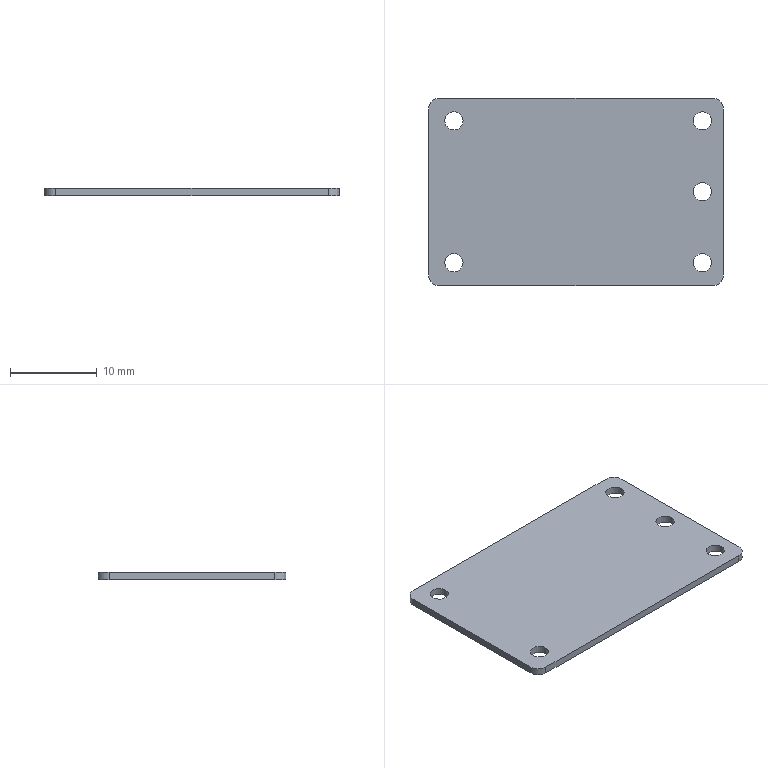Part | STEP file | Driver amplifier PA2PCB | 1 solid | 15 faces | box 34 x 21.66 x 0.832 mm | volume 597.158 mm3 | cylinder 9 | plane 6 | commonest cylinder face diameters 2.1 x5 2.54 x4
STEP:
#1=CARTESIAN_POINT('',(0.,0.,0.));
#2=DIRECTION('',(0.,0.,1.));
#3=DIRECTION('',(1.,0.,0.));
#4=AXIS2_PLACEMENT_3D('',#1,#2,#3);
#5=CARTESIAN_POINT('',(942.668,908.628,0.));
#6=VERTEX_POINT('',#5);
#7=CARTESIAN_POINT('',(942.668,889.508,0.));
#8=VERTEX_POINT('',#7);
#9=CARTESIAN_POINT('',(942.668,908.628,0.));
#10=DIRECTION('',(0.,-1.,0.));
#11=VECTOR('',#10,1.);
#12=LINE('',#9,#11);
#13=CARTESIAN_POINT('',(942.668,908.628,-0.832));
#14=DIRECTION('',(-1.,0.,0.));
#15=DIRECTION('',(0.,0.,1.));
#16=AXIS2_PLACEMENT_3D('',#13,#14,#15);
#17=PLANE('',#16);
#18=CARTESIAN_POINT('',(0.832,0.));
#19=DIRECTION('',(0.,-1.));
#20=VECTOR('',#19,1.);
#21=LINE('',#18,#20);
#22=(GEOMETRIC_REPRESENTATION_CONTEXT(2)PARAMETRIC_REPRESENTATION_CONTEXT()REPRESENTATION_CONTEXT('',''));
#23=DEFINITIONAL_REPRESENTATION('',(#21),#22);
#24=PCURVE('',#17,#23);
#25=CARTESIAN_POINT('',(943.938,889.508,0.));
#26=DIRECTION('',(0.,0.,1.));
#27=DIRECTION('',(1.,0.,0.));
#28=AXIS2_PLACEMENT_3D('',#25,#26,#27);
#29=PLANE('',#28);
#30=CARTESIAN_POINT('',(-1.27,19.12));
#31=DIRECTION('',(0.,-1.));
#32=VECTOR('',#31,1.);
#33=LINE('',#30,#32);
#34=(GEOMETRIC_REPRESENTATION_CONTEXT(2)PARAMETRIC_REPRESENTATION_CONTEXT()REPRESENTATION_CONTEXT('',''));
#35=DEFINITIONAL_REPRESENTATION('',(#33),#34);
#36=PCURVE('',#29,#35);
#37=SURFACE_CURVE('',#12,(#24,#36),.PCURVE_S1.);
#38=EDGE_CURVE('',#6,#8,#37,.T.);
#39=ORIENTED_EDGE('',*,*,#38,.F.);
#40=CARTESIAN_POINT('',(942.668,908.628,-0.832));
#41=VERTEX_POINT('',#40);
#42=CARTESIAN_POINT('',(942.668,908.628,-0.832));
#43=DIRECTION('',(0.,0.,1.));
#44=VECTOR('',#43,1.);
#45=LINE('',#42,#44);
#46=CARTESIAN_POINT('',(0.,0.));
#47=DIRECTION('',(1.,0.));
#48=VECTOR('',#47,1.);
#49=LINE('',#46,#48);
#50=(GEOMETRIC_REPRESENTATION_CONTEXT(2)PARAMETRIC_REPRESENTATION_CONTEXT()REPRESENTATION_CONTEXT('',''));
#51=DEFINITIONAL_REPRESENTATION('',(#49),#50);
#52=PCURVE('',#17,#51);
#53=CARTESIAN_POINT('',(943.938,908.628,-0.832));
#54=DIRECTION('',(0.,0.,1.));
#55=DIRECTION('',(1.,0.,0.));
#56=AXIS2_PLACEMENT_3D('',#53,#54,#55);
#57=CYLINDRICAL_SURFACE('',#56,1.27);
#58=CARTESIAN_POINT('',(3.142,0.));
#59=DIRECTION('',(0.,1.));
#60=VECTOR('',#59,1.);
#61=LINE('',#58,#60);
#62=(GEOMETRIC_REPRESENTATION_CONTEXT(2)PARAMETRIC_REPRESENTATION_CONTEXT()REPRESENTATION_CONTEXT('',''));
#63=DEFINITIONAL_REPRESENTATION('',(#61),#62);
#64=PCURVE('',#57,#63);
#65=SURFACE_CURVE('',#45,(#52,#64),.PCURVE_S1.);
#66=EDGE_CURVE('',#41,#6,#65,.T.);
#67=ORIENTED_EDGE('',*,*,#66,.F.);
#68=CARTESIAN_POINT('',(942.668,889.508,-0.832));
#69=VERTEX_POINT('',#68);
#70=CARTESIAN_POINT('',(942.668,908.628,-0.832));
#71=DIRECTION('',(0.,-1.,0.));
#72=VECTOR('',#71,1.);
#73=LINE('',#70,#72);
#74=CARTESIAN_POINT('',(0.,0.));
#75=DIRECTION('',(0.,-1.));
#76=VECTOR('',#75,1.);
#77=LINE('',#74,#76);
#78=(GEOMETRIC_REPRESENTATION_CONTEXT(2)PARAMETRIC_REPRESENTATION_CONTEXT()REPRESENTATION_CONTEXT('',''));
#79=DEFINITIONAL_REPRESENTATION('',(#77),#78);
#80=PCURVE('',#17,#79);
#81=CARTESIAN_POINT('',(943.938,889.508,-0.832));
#82=DIRECTION('',(0.,0.,1.));
#83=DIRECTION('',(1.,0.,0.));
#84=AXIS2_PLACEMENT_3D('',#81,#82,#83);
#85=PLANE('',#84);
#86=CARTESIAN_POINT('',(-1.27,19.12));
#87=DIRECTION('',(0.,-1.));
#88=VECTOR('',#87,1.);
#89=LINE('',#86,#88);
#90=(GEOMETRIC_REPRESENTATION_CONTEXT(2)PARAMETRIC_REPRESENTATION_CONTEXT()REPRESENTATION_CONTEXT('',''));
#91=DEFINITIONAL_REPRESENTATION('',(#89),#90);
#92=PCURVE('',#85,#91);
#93=SURFACE_CURVE('',#73,(#80,#92),.PCURVE_S1.);
#94=EDGE_CURVE('',#41,#69,#93,.T.);
#95=ORIENTED_EDGE('',*,*,#94,.T.);
#96=CARTESIAN_POINT('',(942.668,889.508,-0.832));
#97=DIRECTION('',(0.,0.,1.));
#98=VECTOR('',#97,1.);
#99=LINE('',#96,#98);
#100=CARTESIAN_POINT('',(0.,-19.12));
#101=DIRECTION('',(1.,0.));
#102=VECTOR('',#101,1.);
#103=LINE('',#100,#102);
#104=(GEOMETRIC_REPRESENTATION_CONTEXT(2)PARAMETRIC_REPRESENTATION_CONTEXT()REPRESENTATION_CONTEXT('',''));
#105=DEFINITIONAL_REPRESENTATION('',(#103),#104);
#106=PCURVE('',#17,#105);
#107=CARTESIAN_POINT('',(943.938,889.508,-0.832));
#108=DIRECTION('',(0.,0.,1.));
#109=DIRECTION('',(1.,0.,0.));
#110=AXIS2_PLACEMENT_3D('',#107,#108,#109);
#111=CYLINDRICAL_SURFACE('',#110,1.27);
#112=CARTESIAN_POINT('',(3.142,0.));
#113=DIRECTION('',(0.,1.));
#114=VECTOR('',#113,1.);
#115=LINE('',#112,#114);
#116=(GEOMETRIC_REPRESENTATION_CONTEXT(2)PARAMETRIC_REPRESENTATION_CONTEXT()REPRESENTATION_CONTEXT('',''));
#117=DEFINITIONAL_REPRESENTATION('',(#115),#116);
#118=PCURVE('',#111,#117);
#119=SURFACE_CURVE('',#99,(#106,#118),.PCURVE_S1.);
#120=EDGE_CURVE('',#69,#8,#119,.T.);
#121=ORIENTED_EDGE('',*,*,#120,.T.);
#122=EDGE_LOOP('',(#39,#67,#95,#121));
#123=FACE_BOUND('',#122,.T.);
#124=ADVANCED_FACE('',(#123),#17,.T.);
#125=CARTESIAN_POINT('',(943.938,888.238,0.));
#126=VERTEX_POINT('',#125);
#127=CARTESIAN_POINT('',(943.938,889.508,0.));
#128=DIRECTION('',(0.,0.,1.));
#129=DIRECTION('',(1.,0.,0.));
#130=AXIS2_PLACEMENT_3D('',#127,#128,#129);
#131=CIRCLE('',#130,1.27);
#132=CARTESIAN_POINT('',(0.,0.832));
#133=DIRECTION('',(1.,0.));
#134=VECTOR('',#133,1.);
#135=LINE('',#132,#134);
#136=(GEOMETRIC_REPRESENTATION_CONTEXT(2)PARAMETRIC_REPRESENTATION_CONTEXT()REPRESENTATION_CONTEXT('',''));
#137=DEFINITIONAL_REPRESENTATION('',(#135),#136);
#138=PCURVE('',#111,#137);
#139=CARTESIAN_POINT('',(0.,0.));
#140=DIRECTION('',(1.,0.));
#141=AXIS2_PLACEMENT_2D('',#139,#140);
#142=CIRCLE('',#141,1.27);
#143=(GEOMETRIC_REPRESENTATION_CONTEXT(2)PARAMETRIC_REPRESENTATION_CONTEXT()REPRESENTATION_CONTEXT('',''));
#144=DEFINITIONAL_REPRESENTATION('',(#142),#143);
#145=PCURVE('',#29,#144);
#146=SURFACE_CURVE('',#131,(#138,#145),.PCURVE_S1.);
#147=EDGE_CURVE('',#8,#126,#146,.T.);
#148=ORIENTED_EDGE('',*,*,#147,.F.);
#149=ORIENTED_EDGE('',*,*,#120,.F.);
#150=CARTESIAN_POINT('',(943.938,888.238,-0.832));
#151=VERTEX_POINT('',#150);
#152=CARTESIAN_POINT('',(943.938,889.508,-0.832));
#153=DIRECTION('',(0.,0.,1.));
#154=DIRECTION('',(1.,0.,0.));
#155=AXIS2_PLACEMENT_3D('',#152,#153,#154);
#156=CIRCLE('',#155,1.27);
#157=CARTESIAN_POINT('',(0.,0.));
#158=DIRECTION('',(1.,0.));
#159=VECTOR('',#158,1.);
#160=LINE('',#157,#159);
#161=(GEOMETRIC_REPRESENTATION_CONTEXT(2)PARAMETRIC_REPRESENTATION_CONTEXT()REPRESENTATION_CONTEXT('',''));
#162=DEFINITIONAL_REPRESENTATION('',(#160),#161);
#163=PCURVE('',#111,#162);
#164=CARTESIAN_POINT('',(0.,0.));
#165=DIRECTION('',(1.,0.));
#166=AXIS2_PLACEMENT_2D('',#164,#165);
#167=CIRCLE('',#166,1.27);
#168=(GEOMETRIC_REPRESENTATION_CONTEXT(2)PARAMETRIC_REPRESENTATION_CONTEXT()REPRESENTATION_CONTEXT('',''));
#169=DEFINITIONAL_REPRESENTATION('',(#167),#168);
#170=PCURVE('',#85,#169);
#171=SURFACE_CURVE('',#156,(#163,#170),.PCURVE_S1.);
#172=EDGE_CURVE('',#69,#151,#171,.T.);
#173=ORIENTED_EDGE('',*,*,#172,.T.);
#174=CARTESIAN_POINT('',(943.938,888.238,-0.832));
#175=DIRECTION('',(0.,0.,1.));
#176=VECTOR('',#175,1.);
#177=LINE('',#174,#176);
#178=CARTESIAN_POINT('',(4.712,0.));
#179=DIRECTION('',(0.,1.));
#180=VECTOR('',#179,1.);
#181=LINE('',#178,#180);
#182=(GEOMETRIC_REPRESENTATION_CONTEXT(2)PARAMETRIC_REPRESENTATION_CONTEXT()REPRESENTATION_CONTEXT('',''));
#183=DEFINITIONAL_REPRESENTATION('',(#181),#182);
#184=PCURVE('',#111,#183);
#185=CARTESIAN_POINT('',(943.938,888.238,-0.832));
#186=DIRECTION('',(0.000000081,-1.,0.));
#187=DIRECTION('',(1.,0.000000081,0.));
#188=AXIS2_PLACEMENT_3D('',#185,#186,#187);
#189=PLANE('',#188);
#190=CARTESIAN_POINT('',(0.,0.));
#191=DIRECTION('',(0.,1.));
#192=VECTOR('',#191,1.);
#193=LINE('',#190,#192);
#194=(GEOMETRIC_REPRESENTATION_CONTEXT(2)PARAMETRIC_REPRESENTATION_CONTEXT()REPRESENTATION_CONTEXT('',''));
#195=DEFINITIONAL_REPRESENTATION('',(#193),#194);
#196=PCURVE('',#189,#195);
#197=SURFACE_CURVE('',#177,(#184,#196),.PCURVE_S1.);
#198=EDGE_CURVE('',#151,#126,#197,.T.);
#199=ORIENTED_EDGE('',*,*,#198,.T.);
#200=EDGE_LOOP('',(#148,#149,#173,#199));
#201=FACE_BOUND('',#200,.T.);
#202=ADVANCED_FACE('',(#201),#111,.T.);
#203=CARTESIAN_POINT('',(975.398,888.238,0.));
#204=VERTEX_POINT('',#203);
#205=CARTESIAN_POINT('',(943.938,888.238,0.));
#206=DIRECTION('',(1.,0.000000081,0.));
#207=VECTOR('',#206,1.);
#208=LINE('',#205,#207);
#209=CARTESIAN_POINT('',(0.,0.832));
#210=DIRECTION('',(1.,0.));
#211=VECTOR('',#210,1.);
#212=LINE('',#209,#211);
#213=(GEOMETRIC_REPRESENTATION_CONTEXT(2)PARAMETRIC_REPRESENTATION_CONTEXT()REPRESENTATION_CONTEXT('',''));
#214=DEFINITIONAL_REPRESENTATION('',(#212),#213);
#215=PCURVE('',#189,#214);
#216=CARTESIAN_POINT('',(0.,-1.27));
#217=DIRECTION('',(1.,0.000000081));
#218=VECTOR('',#217,1.);
#219=LINE('',#216,#218);
#220=(GEOMETRIC_REPRESENTATION_CONTEXT(2)PARAMETRIC_REPRESENTATION_CONTEXT()REPRESENTATION_CONTEXT('',''));
#221=DEFINITIONAL_REPRESENTATION('',(#219),#220);
#222=PCURVE('',#29,#221);
#223=SURFACE_CURVE('',#208,(#215,#222),.PCURVE_S1.);
#224=EDGE_CURVE('',#126,#204,#223,.T.);
#225=ORIENTED_EDGE('',*,*,#224,.F.);
#226=ORIENTED_EDGE('',*,*,#198,.F.);
#227=CARTESIAN_POINT('',(975.398,888.238,-0.832));
#228=VERTEX_POINT('',#227);
#229=CARTESIAN_POINT('',(943.938,888.238,-0.832));
#230=DIRECTION('',(1.,0.000000081,0.));
#231=VECTOR('',#230,1.);
#232=LINE('',#229,#231);
#233=CARTESIAN_POINT('',(0.,0.));
#234=DIRECTION('',(1.,0.));
#235=VECTOR('',#234,1.);
#236=LINE('',#233,#235);
#237=(GEOMETRIC_REPRESENTATION_CONTEXT(2)PARAMETRIC_REPRESENTATION_CONTEXT()REPRESENTATION_CONTEXT('',''));
#238=DEFINITIONAL_REPRESENTATION('',(#236),#237);
#239=PCURVE('',#189,#238);
#240=CARTESIAN_POINT('',(0.,-1.27));
#241=DIRECTION('',(1.,0.000000081));
#242=VECTOR('',#241,1.);
#243=LINE('',#240,#242);
#244=(GEOMETRIC_REPRESENTATION_CONTEXT(2)PARAMETRIC_REPRESENTATION_CONTEXT()REPRESENTATION_CONTEXT('',''));
#245=DEFINITIONAL_REPRESENTATION('',(#243),#244);
#246=PCURVE('',#85,#245);
#247=SURFACE_CURVE('',#232,(#239,#246),.PCURVE_S1.);
#248=EDGE_CURVE('',#151,#228,#247,.T.);
#249=ORIENTED_EDGE('',*,*,#248,.T.);
#250=CARTESIAN_POINT('',(975.398,888.238,-0.832));
#251=DIRECTION('',(0.,0.,1.));
#252=VECTOR('',#251,1.);
#253=LINE('',#250,#252);
#254=CARTESIAN_POINT('',(31.46,0.));
#255=DIRECTION('',(0.,1.));
#256=VECTOR('',#255,1.);
#257=LINE('',#254,#256);
#258=(GEOMETRIC_REPRESENTATION_CONTEXT(2)PARAMETRIC_REPRESENTATION_CONTEXT()REPRESENTATION_CONTEXT('',''));
#259=DEFINITIONAL_REPRESENTATION('',(#257),#258);
#260=PCURVE('',#189,#259);
#261=CARTESIAN_POINT('',(975.398,889.508,-0.832));
#262=DIRECTION('',(0.,0.,1.));
#263=DIRECTION('',(1.,0.,0.));
#264=AXIS2_PLACEMENT_3D('',#261,#262,#263);
#265=CYLINDRICAL_SURFACE('',#264,1.27);
#266=CARTESIAN_POINT('',(4.712,0.));
#267=DIRECTION('',(0.,1.));
#268=VECTOR('',#267,1.);
#269=LINE('',#266,#268);
#270=(GEOMETRIC_REPRESENTATION_CONTEXT(2)PARAMETRIC_REPRESENTATION_CONTEXT()REPRESENTATION_CONTEXT('',''));
#271=DEFINITIONAL_REPRESENTATION('',(#269),#270);
#272=PCURVE('',#265,#271);
#273=SURFACE_CURVE('',#253,(#260,#272),.PCURVE_S1.);
#274=EDGE_CURVE('',#228,#204,#273,.T.);
#275=ORIENTED_EDGE('',*,*,#274,.T.);
#276=EDGE_LOOP('',(#225,#226,#249,#275));
#277=FACE_BOUND('',#276,.T.);
#278=ADVANCED_FACE('',(#277),#189,.T.);
#279=CARTESIAN_POINT('',(976.668,889.508,0.));
#280=VERTEX_POINT('',#279);
#281=CARTESIAN_POINT('',(975.398,889.508,0.));
#282=DIRECTION('',(0.,0.,1.));
#283=DIRECTION('',(1.,0.,0.));
#284=AXIS2_PLACEMENT_3D('',#281,#282,#283);
#285=CIRCLE('',#284,1.27);
#286=CARTESIAN_POINT('',(0.,0.832));
#287=DIRECTION('',(1.,0.));
#288=VECTOR('',#287,1.);
#289=LINE('',#286,#288);
#290=(GEOMETRIC_REPRESENTATION_CONTEXT(2)PARAMETRIC_REPRESENTATION_CONTEXT()REPRESENTATION_CONTEXT('',''));
#291=DEFINITIONAL_REPRESENTATION('',(#289),#290);
#292=PCURVE('',#265,#291);
#293=CARTESIAN_POINT('',(31.46,0.00000254));
#294=DIRECTION('',(1.,0.));
#295=AXIS2_PLACEMENT_2D('',#293,#294);
#296=CIRCLE('',#295,1.27);
#297=(GEOMETRIC_REPRESENTATION_CONTEXT(2)PARAMETRIC_REPRESENTATION_CONTEXT()REPRESENTATION_CONTEXT('',''));
#298=DEFINITIONAL_REPRESENTATION('',(#296),#297);
#299=PCURVE('',#29,#298);
#300=SURFACE_CURVE('',#285,(#292,#299),.PCURVE_S1.);
#301=EDGE_CURVE('',#204,#280,#300,.T.);
#302=ORIENTED_EDGE('',*,*,#301,.F.);
#303=ORIENTED_EDGE('',*,*,#274,.F.);
#304=CARTESIAN_POINT('',(976.668,889.508,-0.832));
#305=VERTEX_POINT('',#304);
#306=CARTESIAN_POINT('',(975.398,889.508,-0.832));
#307=DIRECTION('',(0.,0.,1.));
#308=DIRECTION('',(1.,0.,0.));
#309=AXIS2_PLACEMENT_3D('',#306,#307,#308);
#310=CIRCLE('',#309,1.27);
#311=CARTESIAN_POINT('',(0.,0.));
#312=DIRECTION('',(1.,0.));
#313=VECTOR('',#312,1.);
#314=LINE('',#311,#313);
#315=(GEOMETRIC_REPRESENTATION_CONTEXT(2)PARAMETRIC_REPRESENTATION_CONTEXT()REPRESENTATION_CONTEXT('',''));
#316=DEFINITIONAL_REPRESENTATION('',(#314),#315);
#317=PCURVE('',#265,#316);
#318=CARTESIAN_POINT('',(31.46,0.00000254));
#319=DIRECTION('',(1.,0.));
#320=AXIS2_PLACEMENT_2D('',#318,#319);
#321=CIRCLE('',#320,1.27);
#322=(GEOMETRIC_REPRESENTATION_CONTEXT(2)PARAMETRIC_REPRESENTATION_CONTEXT()REPRESENTATION_CONTEXT('',''));
#323=DEFINITIONAL_REPRESENTATION('',(#321),#322);
#324=PCURVE('',#85,#323);
#325=SURFACE_CURVE('',#310,(#317,#324),.PCURVE_S1.);
#326=EDGE_CURVE('',#228,#305,#325,.T.);
#327=ORIENTED_EDGE('',*,*,#326,.T.);
#328=CARTESIAN_POINT('',(976.668,889.508,-0.832));
#329=DIRECTION('',(0.,0.,1.));
#330=VECTOR('',#329,1.);
#331=LINE('',#328,#330);
#332=CARTESIAN_POINT('',(6.283,0.));
#333=DIRECTION('',(0.,1.));
#334=VECTOR('',#333,1.);
#335=LINE('',#332,#334);
#336=(GEOMETRIC_REPRESENTATION_CONTEXT(2)PARAMETRIC_REPRESENTATION_CONTEXT()REPRESENTATION_CONTEXT('',''));
#337=DEFINITIONAL_REPRESENTATION('',(#335),#336);
#338=PCURVE('',#265,#337);
#339=CARTESIAN_POINT('',(976.668,889.508,-0.832));
#340=DIRECTION('',(1.,0.,0.));
#341=DIRECTION('',(0.,0.,-1.));
#342=AXIS2_PLACEMENT_3D('',#339,#340,#341);
#343=PLANE('',#342);
#344=CARTESIAN_POINT('',(0.,0.));
#345=DIRECTION('',(-1.,0.));
#346=VECTOR('',#345,1.);
#347=LINE('',#344,#346);
#348=(GEOMETRIC_REPRESENTATION_CONTEXT(2)PARAMETRIC_REPRESENTATION_CONTEXT()REPRESENTATION_CONTEXT('',''));
#349=DEFINITIONAL_REPRESENTATION('',(#347),#348);
#350=PCURVE('',#343,#349);
#351=SURFACE_CURVE('',#331,(#338,#350),.PCURVE_S1.);
#352=EDGE_CURVE('',#305,#280,#351,.T.);
#353=ORIENTED_EDGE('',*,*,#352,.T.);
#354=EDGE_LOOP('',(#302,#303,#327,#353));
#355=FACE_BOUND('',#354,.T.);
#356=ADVANCED_FACE('',(#355),#265,.T.);
#357=CARTESIAN_POINT('',(976.668,908.628,0.));
#358=VERTEX_POINT('',#357);
#359=CARTESIAN_POINT('',(976.668,889.508,0.));
#360=DIRECTION('',(0.,1.,0.));
#361=VECTOR('',#360,1.);
#362=LINE('',#359,#361);
#363=CARTESIAN_POINT('',(-0.832,0.));
#364=DIRECTION('',(0.,1.));
#365=VECTOR('',#364,1.);
#366=LINE('',#363,#365);
#367=(GEOMETRIC_REPRESENTATION_CONTEXT(2)PARAMETRIC_REPRESENTATION_CONTEXT()REPRESENTATION_CONTEXT('',''));
#368=DEFINITIONAL_REPRESENTATION('',(#366),#367);
#369=PCURVE('',#343,#368);
#370=CARTESIAN_POINT('',(32.73,0.00000254));
#371=DIRECTION('',(0.,1.));
#372=VECTOR('',#371,1.);
#373=LINE('',#370,#372);
#374=(GEOMETRIC_REPRESENTATION_CONTEXT(2)PARAMETRIC_REPRESENTATION_CONTEXT()REPRESENTATION_CONTEXT('',''));
#375=DEFINITIONAL_REPRESENTATION('',(#373),#374);
#376=PCURVE('',#29,#375);
#377=SURFACE_CURVE('',#362,(#369,#376),.PCURVE_S1.);
#378=EDGE_CURVE('',#280,#358,#377,.T.);
#379=ORIENTED_EDGE('',*,*,#378,.F.);
#380=ORIENTED_EDGE('',*,*,#352,.F.);
#381=CARTESIAN_POINT('',(976.668,908.628,-0.832));
#382=VERTEX_POINT('',#381);
#383=CARTESIAN_POINT('',(976.668,889.508,-0.832));
#384=DIRECTION('',(0.,1.,0.));
#385=VECTOR('',#384,1.);
#386=LINE('',#383,#385);
#387=CARTESIAN_POINT('',(0.,0.));
#388=DIRECTION('',(0.,1.));
#389=VECTOR('',#388,1.);
#390=LINE('',#387,#389);
#391=(GEOMETRIC_REPRESENTATION_CONTEXT(2)PARAMETRIC_REPRESENTATION_CONTEXT()REPRESENTATION_CONTEXT('',''));
#392=DEFINITIONAL_REPRESENTATION('',(#390),#391);
#393=PCURVE('',#343,#392);
#394=CARTESIAN_POINT('',(32.73,0.00000254));
#395=DIRECTION('',(0.,1.));
#396=VECTOR('',#395,1.);
#397=LINE('',#394,#396);
#398=(GEOMETRIC_REPRESENTATION_CONTEXT(2)PARAMETRIC_REPRESENTATION_CONTEXT()REPRESENTATION_CONTEXT('',''));
#399=DEFINITIONAL_REPRESENTATION('',(#397),#398);
#400=PCURVE('',#85,#399);
#401=SURFACE_CURVE('',#386,(#393,#400),.PCURVE_S1.);
#402=EDGE_CURVE('',#305,#382,#401,.T.);
#403=ORIENTED_EDGE('',*,*,#402,.T.);
#404=CARTESIAN_POINT('',(976.668,908.628,-0.832));
#405=DIRECTION('',(0.,0.,1.));
#406=VECTOR('',#405,1.);
#407=LINE('',#404,#406);
#408=CARTESIAN_POINT('',(0.,19.12));
#409=DIRECTION('',(-1.,0.));
#410=VECTOR('',#409,1.);
#411=LINE('',#408,#410);
#412=(GEOMETRIC_REPRESENTATION_CONTEXT(2)PARAMETRIC_REPRESENTATION_CONTEXT()REPRESENTATION_CONTEXT('',''));
#413=DEFINITIONAL_REPRESENTATION('',(#411),#412);
#414=PCURVE('',#343,#413);
#415=CARTESIAN_POINT('',(975.398,908.628,-0.832));
#416=DIRECTION('',(0.,0.,1.));
#417=DIRECTION('',(1.,0.,0.));
#418=AXIS2_PLACEMENT_3D('',#415,#416,#417);
#419=CYLINDRICAL_SURFACE('',#418,1.27);
#420=CARTESIAN_POINT('',(0.,0.));
#421=DIRECTION('',(0.,1.));
#422=VECTOR('',#421,1.);
#423=LINE('',#420,#422);
#424=(GEOMETRIC_REPRESENTATION_CONTEXT(2)PARAMETRIC_REPRESENTATION_CONTEXT()REPRESENTATION_CONTEXT('',''));
#425=DEFINITIONAL_REPRESENTATION('',(#423),#424);
#426=PCURVE('',#419,#425);
#427=SURFACE_CURVE('',#407,(#414,#426),.PCURVE_S1.);
#428=EDGE_CURVE('',#382,#358,#427,.T.);
#429=ORIENTED_EDGE('',*,*,#428,.T.);
#430=EDGE_LOOP('',(#379,#380,#403,#429));
#431=FACE_BOUND('',#430,.T.);
#432=ADVANCED_FACE('',(#431),#343,.T.);
#433=CARTESIAN_POINT('',(975.398,909.898,0.));
#434=VERTEX_POINT('',#433);
#435=CARTESIAN_POINT('',(975.398,908.628,0.));
#436=DIRECTION('',(0.,0.,1.));
#437=DIRECTION('',(1.,0.,0.));
#438=AXIS2_PLACEMENT_3D('',#435,#436,#437);
#439=CIRCLE('',#438,1.27);
#440=CARTESIAN_POINT('',(0.,0.832));
#441=DIRECTION('',(1.,0.));
#442=VECTOR('',#441,1.);
#443=LINE('',#440,#442);
#444=(GEOMETRIC_REPRESENTATION_CONTEXT(2)PARAMETRIC_REPRESENTATION_CONTEXT()REPRESENTATION_CONTEXT('',''));
#445=DEFINITIONAL_REPRESENTATION('',(#443),#444);
#446=PCURVE('',#419,#445);
#447=CARTESIAN_POINT('',(31.46,19.12));
#448=DIRECTION('',(1.,0.));
#449=AXIS2_PLACEMENT_2D('',#447,#448);
#450=CIRCLE('',#449,1.27);
#451=(GEOMETRIC_REPRESENTATION_CONTEXT(2)PARAMETRIC_REPRESENTATION_CONTEXT()REPRESENTATION_CONTEXT('',''));
#452=DEFINITIONAL_REPRESENTATION('',(#450),#451);
#453=PCURVE('',#29,#452);
#454=SURFACE_CURVE('',#439,(#446,#453),.PCURVE_S1.);
#455=EDGE_CURVE('',#358,#434,#454,.T.);
#456=ORIENTED_EDGE('',*,*,#455,.F.);
#457=ORIENTED_EDGE('',*,*,#428,.F.);
#458=CARTESIAN_POINT('',(975.398,909.898,-0.832));
#459=VERTEX_POINT('',#458);
#460=CARTESIAN_POINT('',(975.398,908.628,-0.832));
#461=DIRECTION('',(0.,0.,1.));
#462=DIRECTION('',(1.,0.,0.));
#463=AXIS2_PLACEMENT_3D('',#460,#461,#462);
#464=CIRCLE('',#463,1.27);
#465=CARTESIAN_POINT('',(0.,0.));
#466=DIRECTION('',(1.,0.));
#467=VECTOR('',#466,1.);
#468=LINE('',#465,#467);
#469=(GEOMETRIC_REPRESENTATION_CONTEXT(2)PARAMETRIC_REPRESENTATION_CONTEXT()REPRESENTATION_CONTEXT('',''));
#470=DEFINITIONAL_REPRESENTATION('',(#468),#469);
#471=PCURVE('',#419,#470);
#472=CARTESIAN_POINT('',(31.46,19.12));
#473=DIRECTION('',(1.,0.));
#474=AXIS2_PLACEMENT_2D('',#472,#473);
#475=CIRCLE('',#474,1.27);
#476=(GEOMETRIC_REPRESENTATION_CONTEXT(2)PARAMETRIC_REPRESENTATION_CONTEXT()REPRESENTATION_CONTEXT('',''));
#477=DEFINITIONAL_REPRESENTATION('',(#475),#476);
#478=PCURVE('',#85,#477);
#479=SURFACE_CURVE('',#464,(#471,#478),.PCURVE_S1.);
#480=EDGE_CURVE('',#382,#459,#479,.T.);
#481=ORIENTED_EDGE('',*,*,#480,.T.);
#482=CARTESIAN_POINT('',(975.398,909.898,-0.832));
#483=DIRECTION('',(0.,0.,1.));
#484=VECTOR('',#483,1.);
#485=LINE('',#482,#484);
#486=CARTESIAN_POINT('',(1.571,0.));
#487=DIRECTION('',(0.,1.));
#488=VECTOR('',#487,1.);
#489=LINE('',#486,#488);
#490=(GEOMETRIC_REPRESENTATION_CONTEXT(2)PARAMETRIC_REPRESENTATION_CONTEXT()REPRESENTATION_CONTEXT('',''));
#491=DEFINITIONAL_REPRESENTATION('',(#489),#490);
#492=PCURVE('',#419,#491);
#493=CARTESIAN_POINT('',(975.398,909.898,-0.832));
#494=DIRECTION('',(-0.000000081,1.,0.));
#495=DIRECTION('',(-1.,-0.000000081,0.));
#496=AXIS2_PLACEMENT_3D('',#493,#494,#495);
#497=PLANE('',#496);
#498=CARTESIAN_POINT('',(0.,0.));
#499=DIRECTION('',(0.,1.));
#500=VECTOR('',#499,1.);
#501=LINE('',#498,#500);
#502=(GEOMETRIC_REPRESENTATION_CONTEXT(2)PARAMETRIC_REPRESENTATION_CONTEXT()REPRESENTATION_CONTEXT('',''));
#503=DEFINITIONAL_REPRESENTATION('',(#501),#502);
#504=PCURVE('',#497,#503);
#505=SURFACE_CURVE('',#485,(#492,#504),.PCURVE_S1.);
#506=EDGE_CURVE('',#459,#434,#505,.T.);
#507=ORIENTED_EDGE('',*,*,#506,.T.);
#508=EDGE_LOOP('',(#456,#457,#481,#507));
#509=FACE_BOUND('',#508,.T.);
#510=ADVANCED_FACE('',(#509),#419,.T.);
#511=CARTESIAN_POINT('',(943.938,909.898,0.));
#512=VERTEX_POINT('',#511);
#513=CARTESIAN_POINT('',(975.398,909.898,0.));
#514=DIRECTION('',(-1.,-0.000000081,0.));
#515=VECTOR('',#514,1.);
#516=LINE('',#513,#515);
#517=CARTESIAN_POINT('',(0.,0.832));
#518=DIRECTION('',(1.,0.));
#519=VECTOR('',#518,1.);
#520=LINE('',#517,#519);
#521=(GEOMETRIC_REPRESENTATION_CONTEXT(2)PARAMETRIC_REPRESENTATION_CONTEXT()REPRESENTATION_CONTEXT('',''));
#522=DEFINITIONAL_REPRESENTATION('',(#520),#521);
#523=PCURVE('',#497,#522);
#524=CARTESIAN_POINT('',(31.46,20.39));
#525=DIRECTION('',(-1.,-0.000000081));
#526=VECTOR('',#525,1.);
#527=LINE('',#524,#526);
#528=(GEOMETRIC_REPRESENTATION_CONTEXT(2)PARAMETRIC_REPRESENTATION_CONTEXT()REPRESENTATION_CONTEXT('',''));
#529=DEFINITIONAL_REPRESENTATION('',(#527),#528);
#530=PCURVE('',#29,#529);
#531=SURFACE_CURVE('',#516,(#523,#530),.PCURVE_S1.);
#532=EDGE_CURVE('',#434,#512,#531,.T.);
#533=ORIENTED_EDGE('',*,*,#532,.F.);
#534=ORIENTED_EDGE('',*,*,#506,.F.);
#535=CARTESIAN_POINT('',(943.938,909.898,-0.832));
#536=VERTEX_POINT('',#535);
#537=CARTESIAN_POINT('',(975.398,909.898,-0.832));
#538=DIRECTION('',(-1.,-0.000000081,0.));
#539=VECTOR('',#538,1.);
#540=LINE('',#537,#539);
#541=CARTESIAN_POINT('',(0.,0.));
#542=DIRECTION('',(1.,0.));
#543=VECTOR('',#542,1.);
#544=LINE('',#541,#543);
#545=(GEOMETRIC_REPRESENTATION_CONTEXT(2)PARAMETRIC_REPRESENTATION_CONTEXT()REPRESENTATION_CONTEXT('',''));
#546=DEFINITIONAL_REPRESENTATION('',(#544),#545);
#547=PCURVE('',#497,#546);
#548=CARTESIAN_POINT('',(31.46,20.39));
#549=DIRECTION('',(-1.,-0.000000081));
#550=VECTOR('',#549,1.);
#551=LINE('',#548,#550);
#552=(GEOMETRIC_REPRESENTATION_CONTEXT(2)PARAMETRIC_REPRESENTATION_CONTEXT()REPRESENTATION_CONTEXT('',''));
#553=DEFINITIONAL_REPRESENTATION('',(#551),#552);
#554=PCURVE('',#85,#553);
#555=SURFACE_CURVE('',#540,(#547,#554),.PCURVE_S1.);
#556=EDGE_CURVE('',#459,#536,#555,.T.);
#557=ORIENTED_EDGE('',*,*,#556,.T.);
#558=CARTESIAN_POINT('',(943.938,909.898,-0.832));
#559=DIRECTION('',(0.,0.,1.));
#560=VECTOR('',#559,1.);
#561=LINE('',#558,#560);
#562=CARTESIAN_POINT('',(31.46,0.));
#563=DIRECTION('',(0.,1.));
#564=VECTOR('',#563,1.);
#565=LINE('',#562,#564);
#566=(GEOMETRIC_REPRESENTATION_CONTEXT(2)PARAMETRIC_REPRESENTATION_CONTEXT()REPRESENTATION_CONTEXT('',''));
#567=DEFINITIONAL_REPRESENTATION('',(#565),#566);
#568=PCURVE('',#497,#567);
#569=CARTESIAN_POINT('',(1.571,0.));
#570=DIRECTION('',(0.,1.));
#571=VECTOR('',#570,1.);
#572=LINE('',#569,#571);
#573=(GEOMETRIC_REPRESENTATION_CONTEXT(2)PARAMETRIC_REPRESENTATION_CONTEXT()REPRESENTATION_CONTEXT('',''));
#574=DEFINITIONAL_REPRESENTATION('',(#572),#573);
#575=PCURVE('',#57,#574);
#576=SURFACE_CURVE('',#561,(#568,#575),.PCURVE_S1.);
#577=EDGE_CURVE('',#536,#512,#576,.T.);
#578=ORIENTED_EDGE('',*,*,#577,.T.);
#579=EDGE_LOOP('',(#533,#534,#557,#578));
#580=FACE_BOUND('',#579,.T.);
#581=ADVANCED_FACE('',(#580),#497,.T.);
#582=CARTESIAN_POINT('',(946.638,907.278,-0.832));
#583=VERTEX_POINT('',#582);
#584=CARTESIAN_POINT('',(945.588,907.278,-0.832));
#585=DIRECTION('',(0.,0.,-1.));
#586=DIRECTION('',(1.,0.,0.));
#587=AXIS2_PLACEMENT_3D('',#584,#585,#586);
#588=CIRCLE('',#587,1.05);
#589=CARTESIAN_POINT('',(945.588,907.278,-0.832));
#590=DIRECTION('',(0.,0.,1.));
#591=DIRECTION('',(1.,0.,0.));
#592=AXIS2_PLACEMENT_3D('',#589,#590,#591);
#593=CYLINDRICAL_SURFACE('',#592,1.05);
#594=CARTESIAN_POINT('',(6.283,0.));
#595=DIRECTION('',(-1.,0.));
#596=VECTOR('',#595,1.);
#597=LINE('',#594,#596);
#598=(GEOMETRIC_REPRESENTATION_CONTEXT(2)PARAMETRIC_REPRESENTATION_CONTEXT()REPRESENTATION_CONTEXT('',''));
#599=DEFINITIONAL_REPRESENTATION('',(#597),#598);
#600=PCURVE('',#593,#599);
#601=CARTESIAN_POINT('',(2.7,17.77));
#602=CARTESIAN_POINT('',(2.7,15.951));
#603=CARTESIAN_POINT('',(1.125,16.861));
#604=CARTESIAN_POINT('',(-0.45,17.77));
#605=CARTESIAN_POINT('',(1.125,18.679));
#606=CARTESIAN_POINT('',(2.7,19.589));
#607=CARTESIAN_POINT('',(2.7,17.77));
#608=(BOUNDED_CURVE()B_SPLINE_CURVE(2,(#601,#602,#603,#604,#605,#606,#607),.UNSPECIFIED.,.T.,.F.)B_SPLINE_CURVE_WITH_KNOTS((1,2,2,2,2,1),(-2.094,0.,2.094,4.189,6.283,8.378),.UNSPECIFIED.)CURVE()GEOMETRIC_REPRESENTATION_ITEM()RATIONAL_B_SPLINE_CURVE((1.,0.5,1.,0.5,1.,0.5,1.))REPRESENTATION_ITEM(''));
#609=(GEOMETRIC_REPRESENTATION_CONTEXT(2)PARAMETRIC_REPRESENTATION_CONTEXT()REPRESENTATION_CONTEXT('',''));
#610=DEFINITIONAL_REPRESENTATION('',(#608),#609);
#611=PCURVE('',#85,#610);
#612=SURFACE_CURVE('',#588,(#600,#611),.PCURVE_S1.);
#613=EDGE_CURVE('',#583,#583,#612,.T.);
#614=ORIENTED_EDGE('',*,*,#613,.F.);
#615=CARTESIAN_POINT('',(946.638,907.278,0.));
#616=VERTEX_POINT('',#615);
#617=CARTESIAN_POINT('',(946.638,907.278,-0.832));
#618=CARTESIAN_POINT('',(946.638,907.278,0.));
#619=B_SPLINE_CURVE_WITH_KNOTS('',1,(#617,#618),.UNSPECIFIED.,.F.,.F.,(2,2),(0.,0.832),.PIECEWISE_BEZIER_KNOTS.);
#620=CARTESIAN_POINT('',(6.283,0.));
#621=DIRECTION('',(0.,1.));
#622=VECTOR('',#621,1.);
#623=LINE('',#620,#622);
#624=(GEOMETRIC_REPRESENTATION_CONTEXT(2)PARAMETRIC_REPRESENTATION_CONTEXT()REPRESENTATION_CONTEXT('',''));
#625=DEFINITIONAL_REPRESENTATION('',(#623),#624);
#626=PCURVE('',#593,#625);
#627=CARTESIAN_POINT('',(0.,0.));
#628=DIRECTION('',(0.,1.));
#629=VECTOR('',#628,1.);
#630=LINE('',#627,#629);
#631=(GEOMETRIC_REPRESENTATION_CONTEXT(2)PARAMETRIC_REPRESENTATION_CONTEXT()REPRESENTATION_CONTEXT('',''));
#632=DEFINITIONAL_REPRESENTATION('',(#630),#631);
#633=PCURVE('',#593,#632);
#634=SEAM_CURVE('',#619,(#626,#633),.PCURVE_S1.);
#635=EDGE_CURVE('',#583,#616,#634,.T.);
#636=ORIENTED_EDGE('',*,*,#635,.T.);
#637=CARTESIAN_POINT('',(945.588,907.278,0.));
#638=DIRECTION('',(0.,0.,-1.));
#639=DIRECTION('',(1.,0.,0.));
#640=AXIS2_PLACEMENT_3D('',#637,#638,#639);
#641=CIRCLE('',#640,1.05);
#642=CARTESIAN_POINT('',(6.283,0.832));
#643=DIRECTION('',(-1.,0.));
#644=VECTOR('',#643,1.);
#645=LINE('',#642,#644);
#646=(GEOMETRIC_REPRESENTATION_CONTEXT(2)PARAMETRIC_REPRESENTATION_CONTEXT()REPRESENTATION_CONTEXT('',''));
#647=DEFINITIONAL_REPRESENTATION('',(#645),#646);
#648=PCURVE('',#593,#647);
#649=CARTESIAN_POINT('',(2.7,17.77));
#650=CARTESIAN_POINT('',(2.7,15.951));
#651=CARTESIAN_POINT('',(1.125,16.861));
#652=CARTESIAN_POINT('',(-0.45,17.77));
#653=CARTESIAN_POINT('',(1.125,18.679));
#654=CARTESIAN_POINT('',(2.7,19.589));
#655=CARTESIAN_POINT('',(2.7,17.77));
#656=(BOUNDED_CURVE()B_SPLINE_CURVE(2,(#649,#650,#651,#652,#653,#654,#655),.UNSPECIFIED.,.T.,.F.)B_SPLINE_CURVE_WITH_KNOTS((1,2,2,2,2,1),(-2.094,0.,2.094,4.189,6.283,8.378),.UNSPECIFIED.)CURVE()GEOMETRIC_REPRESENTATION_ITEM()RATIONAL_B_SPLINE_CURVE((1.,0.5,1.,0.5,1.,0.5,1.))REPRESENTATION_ITEM(''));
#657=(GEOMETRIC_REPRESENTATION_CONTEXT(2)PARAMETRIC_REPRESENTATION_CONTEXT()REPRESENTATION_CONTEXT('',''));
#658=DEFINITIONAL_REPRESENTATION('',(#656),#657);
#659=PCURVE('',#29,#658);
#660=SURFACE_CURVE('',#641,(#648,#659),.PCURVE_S1.);
#661=EDGE_CURVE('',#616,#616,#660,.T.);
#662=ORIENTED_EDGE('',*,*,#661,.T.);
#663=ORIENTED_EDGE('',*,*,#635,.F.);
#664=EDGE_LOOP('',(#614,#636,#662,#663));
#665=FACE_BOUND('',#664,.F.);
#666=ADVANCED_FACE('',(#665),#593,.F.);
#667=CARTESIAN_POINT('',(946.638,890.918,-0.832));
#668=VERTEX_POINT('',#667);
#669=CARTESIAN_POINT('',(945.588,890.918,-0.832));
#670=DIRECTION('',(0.,0.,-1.));
#671=DIRECTION('',(1.,0.,0.));
#672=AXIS2_PLACEMENT_3D('',#669,#670,#671);
#673=CIRCLE('',#672,1.05);
#674=CARTESIAN_POINT('',(945.588,890.918,-0.832));
#675=DIRECTION('',(0.,0.,1.));
#676=DIRECTION('',(1.,0.,0.));
#677=AXIS2_PLACEMENT_3D('',#674,#675,#676);
#678=CYLINDRICAL_SURFACE('',#677,1.05);
#679=CARTESIAN_POINT('',(6.283,0.));
#680=DIRECTION('',(-1.,0.));
#681=VECTOR('',#680,1.);
#682=LINE('',#679,#681);
#683=(GEOMETRIC_REPRESENTATION_CONTEXT(2)PARAMETRIC_REPRESENTATION_CONTEXT()REPRESENTATION_CONTEXT('',''));
#684=DEFINITIONAL_REPRESENTATION('',(#682),#683);
#685=PCURVE('',#678,#684);
#686=CARTESIAN_POINT('',(2.7,1.41));
#687=CARTESIAN_POINT('',(2.7,-0.4087));
#688=CARTESIAN_POINT('',(1.125,0.5007));
#689=CARTESIAN_POINT('',(-0.45,1.41));
#690=CARTESIAN_POINT('',(1.125,2.319));
#691=CARTESIAN_POINT('',(2.7,3.229));
#692=CARTESIAN_POINT('',(2.7,1.41));
#693=(BOUNDED_CURVE()B_SPLINE_CURVE(2,(#686,#687,#688,#689,#690,#691,#692),.UNSPECIFIED.,.T.,.F.)B_SPLINE_CURVE_WITH_KNOTS((1,2,2,2,2,1),(-2.094,0.,2.094,4.189,6.283,8.378),.UNSPECIFIED.)CURVE()GEOMETRIC_REPRESENTATION_ITEM()RATIONAL_B_SPLINE_CURVE((1.,0.5,1.,0.5,1.,0.5,1.))REPRESENTATION_ITEM(''));
#694=(GEOMETRIC_REPRESENTATION_CONTEXT(2)PARAMETRIC_REPRESENTATION_CONTEXT()REPRESENTATION_CONTEXT('',''));
#695=DEFINITIONAL_REPRESENTATION('',(#693),#694);
#696=PCURVE('',#85,#695);
#697=SURFACE_CURVE('',#673,(#685,#696),.PCURVE_S1.);
#698=EDGE_CURVE('',#668,#668,#697,.T.);
#699=ORIENTED_EDGE('',*,*,#698,.F.);
#700=CARTESIAN_POINT('',(946.638,890.918,0.));
#701=VERTEX_POINT('',#700);
#702=CARTESIAN_POINT('',(946.638,890.918,-0.832));
#703=CARTESIAN_POINT('',(946.638,890.918,0.));
#704=B_SPLINE_CURVE_WITH_KNOTS('',1,(#702,#703),.UNSPECIFIED.,.F.,.F.,(2,2),(0.,0.832),.PIECEWISE_BEZIER_KNOTS.);
#705=CARTESIAN_POINT('',(6.283,0.));
#706=DIRECTION('',(0.,1.));
#707=VECTOR('',#706,1.);
#708=LINE('',#705,#707);
#709=(GEOMETRIC_REPRESENTATION_CONTEXT(2)PARAMETRIC_REPRESENTATION_CONTEXT()REPRESENTATION_CONTEXT('',''));
#710=DEFINITIONAL_REPRESENTATION('',(#708),#709);
#711=PCURVE('',#678,#710);
#712=CARTESIAN_POINT('',(0.,0.));
#713=DIRECTION('',(0.,1.));
#714=VECTOR('',#713,1.);
#715=LINE('',#712,#714);
#716=(GEOMETRIC_REPRESENTATION_CONTEXT(2)PARAMETRIC_REPRESENTATION_CONTEXT()REPRESENTATION_CONTEXT('',''));
#717=DEFINITIONAL_REPRESENTATION('',(#715),#716);
#718=PCURVE('',#678,#717);
#719=SEAM_CURVE('',#704,(#711,#718),.PCURVE_S1.);
#720=EDGE_CURVE('',#668,#701,#719,.T.);
#721=ORIENTED_EDGE('',*,*,#720,.T.);
#722=CARTESIAN_POINT('',(945.588,890.918,0.));
#723=DIRECTION('',(0.,0.,-1.));
#724=DIRECTION('',(1.,0.,0.));
#725=AXIS2_PLACEMENT_3D('',#722,#723,#724);
#726=CIRCLE('',#725,1.05);
#727=CARTESIAN_POINT('',(6.283,0.832));
#728=DIRECTION('',(-1.,0.));
#729=VECTOR('',#728,1.);
#730=LINE('',#727,#729);
#731=(GEOMETRIC_REPRESENTATION_CONTEXT(2)PARAMETRIC_REPRESENTATION_CONTEXT()REPRESENTATION_CONTEXT('',''));
#732=DEFINITIONAL_REPRESENTATION('',(#730),#731);
#733=PCURVE('',#678,#732);
#734=CARTESIAN_POINT('',(2.7,1.41));
#735=CARTESIAN_POINT('',(2.7,-0.4087));
#736=CARTESIAN_POINT('',(1.125,0.5007));
#737=CARTESIAN_POINT('',(-0.45,1.41));
#738=CARTESIAN_POINT('',(1.125,2.319));
#739=CARTESIAN_POINT('',(2.7,3.229));
#740=CARTESIAN_POINT('',(2.7,1.41));
#741=(BOUNDED_CURVE()B_SPLINE_CURVE(2,(#734,#735,#736,#737,#738,#739,#740),.UNSPECIFIED.,.T.,.F.)B_SPLINE_CURVE_WITH_KNOTS((1,2,2,2,2,1),(-2.094,0.,2.094,4.189,6.283,8.378),.UNSPECIFIED.)CURVE()GEOMETRIC_REPRESENTATION_ITEM()RATIONAL_B_SPLINE_CURVE((1.,0.5,1.,0.5,1.,0.5,1.))REPRESENTATION_ITEM(''));
#742=(GEOMETRIC_REPRESENTATION_CONTEXT(2)PARAMETRIC_REPRESENTATION_CONTEXT()REPRESENTATION_CONTEXT('',''));
#743=DEFINITIONAL_REPRESENTATION('',(#741),#742);
#744=PCURVE('',#29,#743);
#745=SURFACE_CURVE('',#726,(#733,#744),.PCURVE_S1.);
#746=EDGE_CURVE('',#701,#701,#745,.T.);
#747=ORIENTED_EDGE('',*,*,#746,.T.);
#748=ORIENTED_EDGE('',*,*,#720,.F.);
#749=EDGE_LOOP('',(#699,#721,#747,#748));
#750=FACE_BOUND('',#749,.F.);
#751=ADVANCED_FACE('',(#750),#678,.F.);
#752=CARTESIAN_POINT('',(975.278,890.918,-0.832));
#753=VERTEX_POINT('',#752);
#754=CARTESIAN_POINT('',(974.228,890.918,-0.832));
#755=DIRECTION('',(0.,0.,-1.));
#756=DIRECTION('',(1.,0.,0.));
#757=AXIS2_PLACEMENT_3D('',#754,#755,#756);
#758=CIRCLE('',#757,1.05);
#759=CARTESIAN_POINT('',(974.228,890.918,-0.832));
#760=DIRECTION('',(0.,0.,1.));
#761=DIRECTION('',(1.,0.,0.));
#762=AXIS2_PLACEMENT_3D('',#759,#760,#761);
#763=CYLINDRICAL_SURFACE('',#762,1.05);
#764=CARTESIAN_POINT('',(6.283,0.));
#765=DIRECTION('',(-1.,0.));
#766=VECTOR('',#765,1.);
#767=LINE('',#764,#766);
#768=(GEOMETRIC_REPRESENTATION_CONTEXT(2)PARAMETRIC_REPRESENTATION_CONTEXT()REPRESENTATION_CONTEXT('',''));
#769=DEFINITIONAL_REPRESENTATION('',(#767),#768);
#770=PCURVE('',#763,#769);
#771=CARTESIAN_POINT('',(31.34,1.41));
#772=CARTESIAN_POINT('',(31.34,-0.4087));
#773=CARTESIAN_POINT('',(29.765,0.5007));
#774=CARTESIAN_POINT('',(28.19,1.41));
#775=CARTESIAN_POINT('',(29.765,2.319));
#776=CARTESIAN_POINT('',(31.34,3.229));
#777=CARTESIAN_POINT('',(31.34,1.41));
#778=(BOUNDED_CURVE()B_SPLINE_CURVE(2,(#771,#772,#773,#774,#775,#776,#777),.UNSPECIFIED.,.T.,.F.)B_SPLINE_CURVE_WITH_KNOTS((1,2,2,2,2,1),(-2.094,0.,2.094,4.189,6.283,8.378),.UNSPECIFIED.)CURVE()GEOMETRIC_REPRESENTATION_ITEM()RATIONAL_B_SPLINE_CURVE((1.,0.5,1.,0.5,1.,0.5,1.))REPRESENTATION_ITEM(''));
#779=(GEOMETRIC_REPRESENTATION_CONTEXT(2)PARAMETRIC_REPRESENTATION_CONTEXT()REPRESENTATION_CONTEXT('',''));
#780=DEFINITIONAL_REPRESENTATION('',(#778),#779);
#781=PCURVE('',#85,#780);
#782=SURFACE_CURVE('',#758,(#770,#781),.PCURVE_S1.);
#783=EDGE_CURVE('',#753,#753,#782,.T.);
#784=ORIENTED_EDGE('',*,*,#783,.F.);
#785=CARTESIAN_POINT('',(975.278,890.918,0.));
#786=VERTEX_POINT('',#785);
#787=CARTESIAN_POINT('',(975.278,890.918,-0.832));
#788=CARTESIAN_POINT('',(975.278,890.918,0.));
#789=B_SPLINE_CURVE_WITH_KNOTS('',1,(#787,#788),.UNSPECIFIED.,.F.,.F.,(2,2),(0.,0.832),.PIECEWISE_BEZIER_KNOTS.);
#790=CARTESIAN_POINT('',(6.283,0.));
#791=DIRECTION('',(0.,1.));
#792=VECTOR('',#791,1.);
#793=LINE('',#790,#792);
#794=(GEOMETRIC_REPRESENTATION_CONTEXT(2)PARAMETRIC_REPRESENTATION_CONTEXT()REPRESENTATION_CONTEXT('',''));
#795=DEFINITIONAL_REPRESENTATION('',(#793),#794);
#796=PCURVE('',#763,#795);
#797=CARTESIAN_POINT('',(0.,0.));
#798=DIRECTION('',(0.,1.));
#799=VECTOR('',#798,1.);
#800=LINE('',#797,#799);
#801=(GEOMETRIC_REPRESENTATION_CONTEXT(2)PARAMETRIC_REPRESENTATION_CONTEXT()REPRESENTATION_CONTEXT('',''));
#802=DEFINITIONAL_REPRESENTATION('',(#800),#801);
#803=PCURVE('',#763,#802);
#804=SEAM_CURVE('',#789,(#796,#803),.PCURVE_S1.);
#805=EDGE_CURVE('',#753,#786,#804,.T.);
#806=ORIENTED_EDGE('',*,*,#805,.T.);
#807=CARTESIAN_POINT('',(974.228,890.918,0.));
#808=DIRECTION('',(0.,0.,-1.));
#809=DIRECTION('',(1.,0.,0.));
#810=AXIS2_PLACEMENT_3D('',#807,#808,#809);
#811=CIRCLE('',#810,1.05);
#812=CARTESIAN_POINT('',(6.283,0.832));
#813=DIRECTION('',(-1.,0.));
#814=VECTOR('',#813,1.);
#815=LINE('',#812,#814);
#816=(GEOMETRIC_REPRESENTATION_CONTEXT(2)PARAMETRIC_REPRESENTATION_CONTEXT()REPRESENTATION_CONTEXT('',''));
#817=DEFINITIONAL_REPRESENTATION('',(#815),#816);
#818=PCURVE('',#763,#817);
#819=CARTESIAN_POINT('',(31.34,1.41));
#820=CARTESIAN_POINT('',(31.34,-0.4087));
#821=CARTESIAN_POINT('',(29.765,0.5007));
#822=CARTESIAN_POINT('',(28.19,1.41));
#823=CARTESIAN_POINT('',(29.765,2.319));
#824=CARTESIAN_POINT('',(31.34,3.229));
#825=CARTESIAN_POINT('',(31.34,1.41));
#826=(BOUNDED_CURVE()B_SPLINE_CURVE(2,(#819,#820,#821,#822,#823,#824,#825),.UNSPECIFIED.,.T.,.F.)B_SPLINE_CURVE_WITH_KNOTS((1,2,2,2,2,1),(-2.094,0.,2.094,4.189,6.283,8.378),.UNSPECIFIED.)CURVE()GEOMETRIC_REPRESENTATION_ITEM()RATIONAL_B_SPLINE_CURVE((1.,0.5,1.,0.5,1.,0.5,1.))REPRESENTATION_ITEM(''));
#827=(GEOMETRIC_REPRESENTATION_CONTEXT(2)PARAMETRIC_REPRESENTATION_CONTEXT()REPRESENTATION_CONTEXT('',''));
#828=DEFINITIONAL_REPRESENTATION('',(#826),#827);
#829=PCURVE('',#29,#828);
#830=SURFACE_CURVE('',#811,(#818,#829),.PCURVE_S1.);
#831=EDGE_CURVE('',#786,#786,#830,.T.);
#832=ORIENTED_EDGE('',*,*,#831,.T.);
#833=ORIENTED_EDGE('',*,*,#805,.F.);
#834=EDGE_LOOP('',(#784,#806,#832,#833));
#835=FACE_BOUND('',#834,.F.);
#836=ADVANCED_FACE('',(#835),#763,.F.);
#837=CARTESIAN_POINT('',(975.278,907.278,-0.832));
#838=VERTEX_POINT('',#837);
#839=CARTESIAN_POINT('',(974.228,907.278,-0.832));
#840=DIRECTION('',(0.,0.,-1.));
#841=DIRECTION('',(1.,0.,0.));
#842=AXIS2_PLACEMENT_3D('',#839,#840,#841);
#843=CIRCLE('',#842,1.05);
#844=CARTESIAN_POINT('',(974.228,907.278,-0.832));
#845=DIRECTION('',(0.,0.,1.));
#846=DIRECTION('',(1.,0.,0.));
#847=AXIS2_PLACEMENT_3D('',#844,#845,#846);
#848=CYLINDRICAL_SURFACE('',#847,1.05);
#849=CARTESIAN_POINT('',(6.283,0.));
#850=DIRECTION('',(-1.,0.));
#851=VECTOR('',#850,1.);
#852=LINE('',#849,#851);
#853=(GEOMETRIC_REPRESENTATION_CONTEXT(2)PARAMETRIC_REPRESENTATION_CONTEXT()REPRESENTATION_CONTEXT('',''));
#854=DEFINITIONAL_REPRESENTATION('',(#852),#853);
#855=PCURVE('',#848,#854);
#856=CARTESIAN_POINT('',(31.34,17.77));
#857=CARTESIAN_POINT('',(31.34,15.951));
#858=CARTESIAN_POINT('',(29.765,16.861));
#859=CARTESIAN_POINT('',(28.19,17.77));
#860=CARTESIAN_POINT('',(29.765,18.679));
#861=CARTESIAN_POINT('',(31.34,19.589));
#862=CARTESIAN_POINT('',(31.34,17.77));
#863=(BOUNDED_CURVE()B_SPLINE_CURVE(2,(#856,#857,#858,#859,#860,#861,#862),.UNSPECIFIED.,.T.,.F.)B_SPLINE_CURVE_WITH_KNOTS((1,2,2,2,2,1),(-2.094,0.,2.094,4.189,6.283,8.378),.UNSPECIFIED.)CURVE()GEOMETRIC_REPRESENTATION_ITEM()RATIONAL_B_SPLINE_CURVE((1.,0.5,1.,0.5,1.,0.5,1.))REPRESENTATION_ITEM(''));
#864=(GEOMETRIC_REPRESENTATION_CONTEXT(2)PARAMETRIC_REPRESENTATION_CONTEXT()REPRESENTATION_CONTEXT('',''));
#865=DEFINITIONAL_REPRESENTATION('',(#863),#864);
#866=PCURVE('',#85,#865);
#867=SURFACE_CURVE('',#843,(#855,#866),.PCURVE_S1.);
#868=EDGE_CURVE('',#838,#838,#867,.T.);
#869=ORIENTED_EDGE('',*,*,#868,.F.);
#870=CARTESIAN_POINT('',(975.278,907.278,0.));
#871=VERTEX_POINT('',#870);
#872=CARTESIAN_POINT('',(975.278,907.278,-0.832));
#873=CARTESIAN_POINT('',(975.278,907.278,0.));
#874=B_SPLINE_CURVE_WITH_KNOTS('',1,(#872,#873),.UNSPECIFIED.,.F.,.F.,(2,2),(0.,0.832),.PIECEWISE_BEZIER_KNOTS.);
#875=CARTESIAN_POINT('',(6.283,0.));
#876=DIRECTION('',(0.,1.));
#877=VECTOR('',#876,1.);
#878=LINE('',#875,#877);
#879=(GEOMETRIC_REPRESENTATION_CONTEXT(2)PARAMETRIC_REPRESENTATION_CONTEXT()REPRESENTATION_CONTEXT('',''));
#880=DEFINITIONAL_REPRESENTATION('',(#878),#879);
#881=PCURVE('',#848,#880);
#882=CARTESIAN_POINT('',(0.,0.));
#883=DIRECTION('',(0.,1.));
#884=VECTOR('',#883,1.);
#885=LINE('',#882,#884);
#886=(GEOMETRIC_REPRESENTATION_CONTEXT(2)PARAMETRIC_REPRESENTATION_CONTEXT()REPRESENTATION_CONTEXT('',''));
#887=DEFINITIONAL_REPRESENTATION('',(#885),#886);
#888=PCURVE('',#848,#887);
#889=SEAM_CURVE('',#874,(#881,#888),.PCURVE_S1.);
#890=EDGE_CURVE('',#838,#871,#889,.T.);
#891=ORIENTED_EDGE('',*,*,#890,.T.);
#892=CARTESIAN_POINT('',(974.228,907.278,0.));
#893=DIRECTION('',(0.,0.,-1.));
#894=DIRECTION('',(1.,0.,0.));
#895=AXIS2_PLACEMENT_3D('',#892,#893,#894);
#896=CIRCLE('',#895,1.05);
#897=CARTESIAN_POINT('',(6.283,0.832));
#898=DIRECTION('',(-1.,0.));
#899=VECTOR('',#898,1.);
#900=LINE('',#897,#899);
#901=(GEOMETRIC_REPRESENTATION_CONTEXT(2)PARAMETRIC_REPRESENTATION_CONTEXT()REPRESENTATION_CONTEXT('',''));
#902=DEFINITIONAL_REPRESENTATION('',(#900),#901);
#903=PCURVE('',#848,#902);
#904=CARTESIAN_POINT('',(31.34,17.77));
#905=CARTESIAN_POINT('',(31.34,15.951));
#906=CARTESIAN_POINT('',(29.765,16.861));
#907=CARTESIAN_POINT('',(28.19,17.77));
#908=CARTESIAN_POINT('',(29.765,18.679));
#909=CARTESIAN_POINT('',(31.34,19.589));
#910=CARTESIAN_POINT('',(31.34,17.77));
#911=(BOUNDED_CURVE()B_SPLINE_CURVE(2,(#904,#905,#906,#907,#908,#909,#910),.UNSPECIFIED.,.T.,.F.)B_SPLINE_CURVE_WITH_KNOTS((1,2,2,2,2,1),(-2.094,0.,2.094,4.189,6.283,8.378),.UNSPECIFIED.)CURVE()GEOMETRIC_REPRESENTATION_ITEM()RATIONAL_B_SPLINE_CURVE((1.,0.5,1.,0.5,1.,0.5,1.))REPRESENTATION_ITEM(''));
#912=(GEOMETRIC_REPRESENTATION_CONTEXT(2)PARAMETRIC_REPRESENTATION_CONTEXT()REPRESENTATION_CONTEXT('',''));
#913=DEFINITIONAL_REPRESENTATION('',(#911),#912);
#914=PCURVE('',#29,#913);
#915=SURFACE_CURVE('',#896,(#903,#914),.PCURVE_S1.);
#916=EDGE_CURVE('',#871,#871,#915,.T.);
#917=ORIENTED_EDGE('',*,*,#916,.T.);
#918=ORIENTED_EDGE('',*,*,#890,.F.);
#919=EDGE_LOOP('',(#869,#891,#917,#918));
#920=FACE_BOUND('',#919,.F.);
#921=ADVANCED_FACE('',(#920),#848,.F.);
#922=CARTESIAN_POINT('',(943.938,908.628,0.));
#923=DIRECTION('',(0.,0.,1.));
#924=DIRECTION('',(1.,0.,0.));
#925=AXIS2_PLACEMENT_3D('',#922,#923,#924);
#926=CIRCLE('',#925,1.27);
#927=CARTESIAN_POINT('',(0.,0.832));
#928=DIRECTION('',(1.,0.));
#929=VECTOR('',#928,1.);
#930=LINE('',#927,#929);
#931=(GEOMETRIC_REPRESENTATION_CONTEXT(2)PARAMETRIC_REPRESENTATION_CONTEXT()REPRESENTATION_CONTEXT('',''));
#932=DEFINITIONAL_REPRESENTATION('',(#930),#931);
#933=PCURVE('',#57,#932);
#934=CARTESIAN_POINT('',(0.,19.12));
#935=DIRECTION('',(1.,0.));
#936=AXIS2_PLACEMENT_2D('',#934,#935);
#937=CIRCLE('',#936,1.27);
#938=(GEOMETRIC_REPRESENTATION_CONTEXT(2)PARAMETRIC_REPRESENTATION_CONTEXT()REPRESENTATION_CONTEXT('',''));
#939=DEFINITIONAL_REPRESENTATION('',(#937),#938);
#940=PCURVE('',#29,#939);
#941=SURFACE_CURVE('',#926,(#933,#940),.PCURVE_S1.);
#942=EDGE_CURVE('',#512,#6,#941,.T.);
#943=ORIENTED_EDGE('',*,*,#942,.F.);
#944=ORIENTED_EDGE('',*,*,#577,.F.);
#945=CARTESIAN_POINT('',(943.938,908.628,-0.832));
#946=DIRECTION('',(0.,0.,1.));
#947=DIRECTION('',(1.,0.,0.));
#948=AXIS2_PLACEMENT_3D('',#945,#946,#947);
#949=CIRCLE('',#948,1.27);
#950=CARTESIAN_POINT('',(0.,0.));
#951=DIRECTION('',(1.,0.));
#952=VECTOR('',#951,1.);
#953=LINE('',#950,#952);
#954=(GEOMETRIC_REPRESENTATION_CONTEXT(2)PARAMETRIC_REPRESENTATION_CONTEXT()REPRESENTATION_CONTEXT('',''));
#955=DEFINITIONAL_REPRESENTATION('',(#953),#954);
#956=PCURVE('',#57,#955);
#957=CARTESIAN_POINT('',(0.,19.12));
#958=DIRECTION('',(1.,0.));
#959=AXIS2_PLACEMENT_2D('',#957,#958);
#960=CIRCLE('',#959,1.27);
#961=(GEOMETRIC_REPRESENTATION_CONTEXT(2)PARAMETRIC_REPRESENTATION_CONTEXT()REPRESENTATION_CONTEXT('',''));
#962=DEFINITIONAL_REPRESENTATION('',(#960),#961);
#963=PCURVE('',#85,#962);
#964=SURFACE_CURVE('',#949,(#956,#963),.PCURVE_S1.);
#965=EDGE_CURVE('',#536,#41,#964,.T.);
#966=ORIENTED_EDGE('',*,*,#965,.T.);
#967=ORIENTED_EDGE('',*,*,#66,.T.);
#968=EDGE_LOOP('',(#943,#944,#966,#967));
#969=FACE_BOUND('',#968,.T.);
#970=ADVANCED_FACE('',(#969),#57,.T.);
#971=CARTESIAN_POINT('',(975.278,899.098,-0.832));
#972=VERTEX_POINT('',#971);
#973=CARTESIAN_POINT('',(974.228,899.098,-0.832));
#974=DIRECTION('',(0.,0.,-1.));
#975=DIRECTION('',(1.,0.,0.));
#976=AXIS2_PLACEMENT_3D('',#973,#974,#975);
#977=CIRCLE('',#976,1.05);
#978=CARTESIAN_POINT('',(974.228,899.098,-0.832));
#979=DIRECTION('',(0.,0.,1.));
#980=DIRECTION('',(1.,0.,0.));
#981=AXIS2_PLACEMENT_3D('',#978,#979,#980);
#982=CYLINDRICAL_SURFACE('',#981,1.05);
#983=CARTESIAN_POINT('',(6.283,0.));
#984=DIRECTION('',(-1.,0.));
#985=VECTOR('',#984,1.);
#986=LINE('',#983,#985);
#987=(GEOMETRIC_REPRESENTATION_CONTEXT(2)PARAMETRIC_REPRESENTATION_CONTEXT()REPRESENTATION_CONTEXT('',''));
#988=DEFINITIONAL_REPRESENTATION('',(#986),#987);
#989=PCURVE('',#982,#988);
#990=CARTESIAN_POINT('',(31.34,9.59));
#991=CARTESIAN_POINT('',(31.34,7.771));
#992=CARTESIAN_POINT('',(29.765,8.681));
#993=CARTESIAN_POINT('',(28.19,9.59));
#994=CARTESIAN_POINT('',(29.765,10.499));
#995=CARTESIAN_POINT('',(31.34,11.409));
#996=CARTESIAN_POINT('',(31.34,9.59));
#997=(BOUNDED_CURVE()B_SPLINE_CURVE(2,(#990,#991,#992,#993,#994,#995,#996),.UNSPECIFIED.,.T.,.F.)B_SPLINE_CURVE_WITH_KNOTS((1,2,2,2,2,1),(-2.094,0.,2.094,4.189,6.283,8.378),.UNSPECIFIED.)CURVE()GEOMETRIC_REPRESENTATION_ITEM()RATIONAL_B_SPLINE_CURVE((1.,0.5,1.,0.5,1.,0.5,1.))REPRESENTATION_ITEM(''));
#998=(GEOMETRIC_REPRESENTATION_CONTEXT(2)PARAMETRIC_REPRESENTATION_CONTEXT()REPRESENTATION_CONTEXT('',''));
#999=DEFINITIONAL_REPRESENTATION('',(#997),#998);
#1000=PCURVE('',#85,#999);
#1001=SURFACE_CURVE('',#977,(#989,#1000),.PCURVE_S1.);
#1002=EDGE_CURVE('',#972,#972,#1001,.T.);
#1003=ORIENTED_EDGE('',*,*,#1002,.F.);
#1004=CARTESIAN_POINT('',(975.278,899.098,0.));
#1005=VERTEX_POINT('',#1004);
#1006=CARTESIAN_POINT('',(975.278,899.098,-0.832));
#1007=CARTESIAN_POINT('',(975.278,899.098,0.));
#1008=B_SPLINE_CURVE_WITH_KNOTS('',1,(#1006,#1007),.UNSPECIFIED.,.F.,.F.,(2,2),(0.,0.832),.PIECEWISE_BEZIER_KNOTS.);
#1009=CARTESIAN_POINT('',(6.283,0.));
#1010=DIRECTION('',(0.,1.));
#1011=VECTOR('',#1010,1.);
#1012=LINE('',#1009,#1011);
#1013=(GEOMETRIC_REPRESENTATION_CONTEXT(2)PARAMETRIC_REPRESENTATION_CONTEXT()REPRESENTATION_CONTEXT('',''));
#1014=DEFINITIONAL_REPRESENTATION('',(#1012),#1013);
#1015=PCURVE('',#982,#1014);
#1016=CARTESIAN_POINT('',(0.,0.));
#1017=DIRECTION('',(0.,1.));
#1018=VECTOR('',#1017,1.);
#1019=LINE('',#1016,#1018);
#1020=(GEOMETRIC_REPRESENTATION_CONTEXT(2)PARAMETRIC_REPRESENTATION_CONTEXT()REPRESENTATION_CONTEXT('',''));
#1021=DEFINITIONAL_REPRESENTATION('',(#1019),#1020);
#1022=PCURVE('',#982,#1021);
#1023=SEAM_CURVE('',#1008,(#1015,#1022),.PCURVE_S1.);
#1024=EDGE_CURVE('',#972,#1005,#1023,.T.);
#1025=ORIENTED_EDGE('',*,*,#1024,.T.);
#1026=CARTESIAN_POINT('',(974.228,899.098,0.));
#1027=DIRECTION('',(0.,0.,-1.));
#1028=DIRECTION('',(1.,0.,0.));
#1029=AXIS2_PLACEMENT_3D('',#1026,#1027,#1028);
#1030=CIRCLE('',#1029,1.05);
#1031=CARTESIAN_POINT('',(6.283,0.832));
#1032=DIRECTION('',(-1.,0.));
#1033=VECTOR('',#1032,1.);
#1034=LINE('',#1031,#1033);
#1035=(GEOMETRIC_REPRESENTATION_CONTEXT(2)PARAMETRIC_REPRESENTATION_CONTEXT()REPRESENTATION_CONTEXT('',''));
#1036=DEFINITIONAL_REPRESENTATION('',(#1034),#1035);
#1037=PCURVE('',#982,#1036);
#1038=CARTESIAN_POINT('',(31.34,9.59));
#1039=CARTESIAN_POINT('',(31.34,7.771));
#1040=CARTESIAN_POINT('',(29.765,8.681));
#1041=CARTESIAN_POINT('',(28.19,9.59));
#1042=CARTESIAN_POINT('',(29.765,10.499));
#1043=CARTESIAN_POINT('',(31.34,11.409));
#1044=CARTESIAN_POINT('',(31.34,9.59));
#1045=(BOUNDED_CURVE()B_SPLINE_CURVE(2,(#1038,#1039,#1040,#1041,#1042,#1043,#1044),.UNSPECIFIED.,.T.,.F.)B_SPLINE_CURVE_WITH_KNOTS((1,2,2,2,2,1),(-2.094,0.,2.094,4.189,6.283,8.378),.UNSPECIFIED.)CURVE()GEOMETRIC_REPRESENTATION_ITEM()RATIONAL_B_SPLINE_CURVE((1.,0.5,1.,0.5,1.,0.5,1.))REPRESENTATION_ITEM(''));
#1046=(GEOMETRIC_REPRESENTATION_CONTEXT(2)PARAMETRIC_REPRESENTATION_CONTEXT()REPRESENTATION_CONTEXT('',''));
#1047=DEFINITIONAL_REPRESENTATION('',(#1045),#1046);
#1048=PCURVE('',#29,#1047);
#1049=SURFACE_CURVE('',#1030,(#1037,#1048),.PCURVE_S1.);
#1050=EDGE_CURVE('',#1005,#1005,#1049,.T.);
#1051=ORIENTED_EDGE('',*,*,#1050,.T.);
#1052=ORIENTED_EDGE('',*,*,#1024,.F.);
#1053=EDGE_LOOP('',(#1003,#1025,#1051,#1052));
#1054=FACE_BOUND('',#1053,.F.);
#1055=ADVANCED_FACE('',(#1054),#982,.F.);
#1056=ORIENTED_EDGE('',*,*,#94,.F.);
#1057=ORIENTED_EDGE('',*,*,#965,.F.);
#1058=ORIENTED_EDGE('',*,*,#556,.F.);
#1059=ORIENTED_EDGE('',*,*,#480,.F.);
#1060=ORIENTED_EDGE('',*,*,#402,.F.);
#1061=ORIENTED_EDGE('',*,*,#326,.F.);
#1062=ORIENTED_EDGE('',*,*,#248,.F.);
#1063=ORIENTED_EDGE('',*,*,#172,.F.);
#1064=EDGE_LOOP('',(#1056,#1057,#1058,#1059,#1060,#1061,#1062,#1063));
#1065=FACE_BOUND('',#1064,.T.);
#1066=ORIENTED_EDGE('',*,*,#868,.F.);
#1067=EDGE_LOOP('',(#1066));
#1068=FACE_BOUND('',#1067,.T.);
#1069=ORIENTED_EDGE('',*,*,#783,.F.);
#1070=EDGE_LOOP('',(#1069));
#1071=FACE_BOUND('',#1070,.T.);
#1072=ORIENTED_EDGE('',*,*,#698,.F.);
#1073=EDGE_LOOP('',(#1072));
#1074=FACE_BOUND('',#1073,.T.);
#1075=ORIENTED_EDGE('',*,*,#613,.F.);
#1076=EDGE_LOOP('',(#1075));
#1077=FACE_BOUND('',#1076,.T.);
#1078=ORIENTED_EDGE('',*,*,#1002,.F.);
#1079=EDGE_LOOP('',(#1078));
#1080=FACE_BOUND('',#1079,.T.);
#1081=ADVANCED_FACE('',(#1065,#1068,#1071,#1074,#1077,#1080),#85,.F.);
#1082=ORIENTED_EDGE('',*,*,#38,.T.);
#1083=ORIENTED_EDGE('',*,*,#147,.T.);
#1084=ORIENTED_EDGE('',*,*,#224,.T.);
#1085=ORIENTED_EDGE('',*,*,#301,.T.);
#1086=ORIENTED_EDGE('',*,*,#378,.T.);
#1087=ORIENTED_EDGE('',*,*,#455,.T.);
#1088=ORIENTED_EDGE('',*,*,#532,.T.);
#1089=ORIENTED_EDGE('',*,*,#942,.T.);
#1090=EDGE_LOOP('',(#1082,#1083,#1084,#1085,#1086,#1087,#1088,#1089));
#1091=FACE_BOUND('',#1090,.T.);
#1092=ORIENTED_EDGE('',*,*,#916,.T.);
#1093=EDGE_LOOP('',(#1092));
#1094=FACE_BOUND('',#1093,.T.);
#1095=ORIENTED_EDGE('',*,*,#831,.T.);
#1096=EDGE_LOOP('',(#1095));
#1097=FACE_BOUND('',#1096,.T.);
#1098=ORIENTED_EDGE('',*,*,#746,.T.);
#1099=EDGE_LOOP('',(#1098));
#1100=FACE_BOUND('',#1099,.T.);
#1101=ORIENTED_EDGE('',*,*,#661,.T.);
#1102=EDGE_LOOP('',(#1101));
#1103=FACE_BOUND('',#1102,.T.);
#1104=ORIENTED_EDGE('',*,*,#1050,.T.);
#1105=EDGE_LOOP('',(#1104));
#1106=FACE_BOUND('',#1105,.T.);
#1107=ADVANCED_FACE('',(#1091,#1094,#1097,#1100,#1103,#1106),#29,.T.);
#1108=CLOSED_SHELL('',(#124,#202,#278,#356,#432,#510,#581,#666,#751,#836,#921,#970,#1055,#1081,#1107));
#1109=MANIFOLD_SOLID_BREP('',#1108);
#1110=(LENGTH_UNIT()NAMED_UNIT(*)SI_UNIT(.MILLI.,.METRE.));
#1111=UNCERTAINTY_MEASURE_WITH_UNIT(LENGTH_MEASURE(0.000002),#1110,'','');
#1112=(NAMED_UNIT(*)PLANE_ANGLE_UNIT()SI_UNIT($,.RADIAN.));
#1113=(NAMED_UNIT(*)SI_UNIT($,.STERADIAN.)SOLID_ANGLE_UNIT());
#1114=(GEOMETRIC_REPRESENTATION_CONTEXT(3)GLOBAL_UNCERTAINTY_ASSIGNED_CONTEXT((#1111))GLOBAL_UNIT_ASSIGNED_CONTEXT((#1110,#1112,#1113))REPRESENTATION_CONTEXT('',''));
#1115=ADVANCED_BREP_SHAPE_REPRESENTATION('',(#4,#1109),#1114);